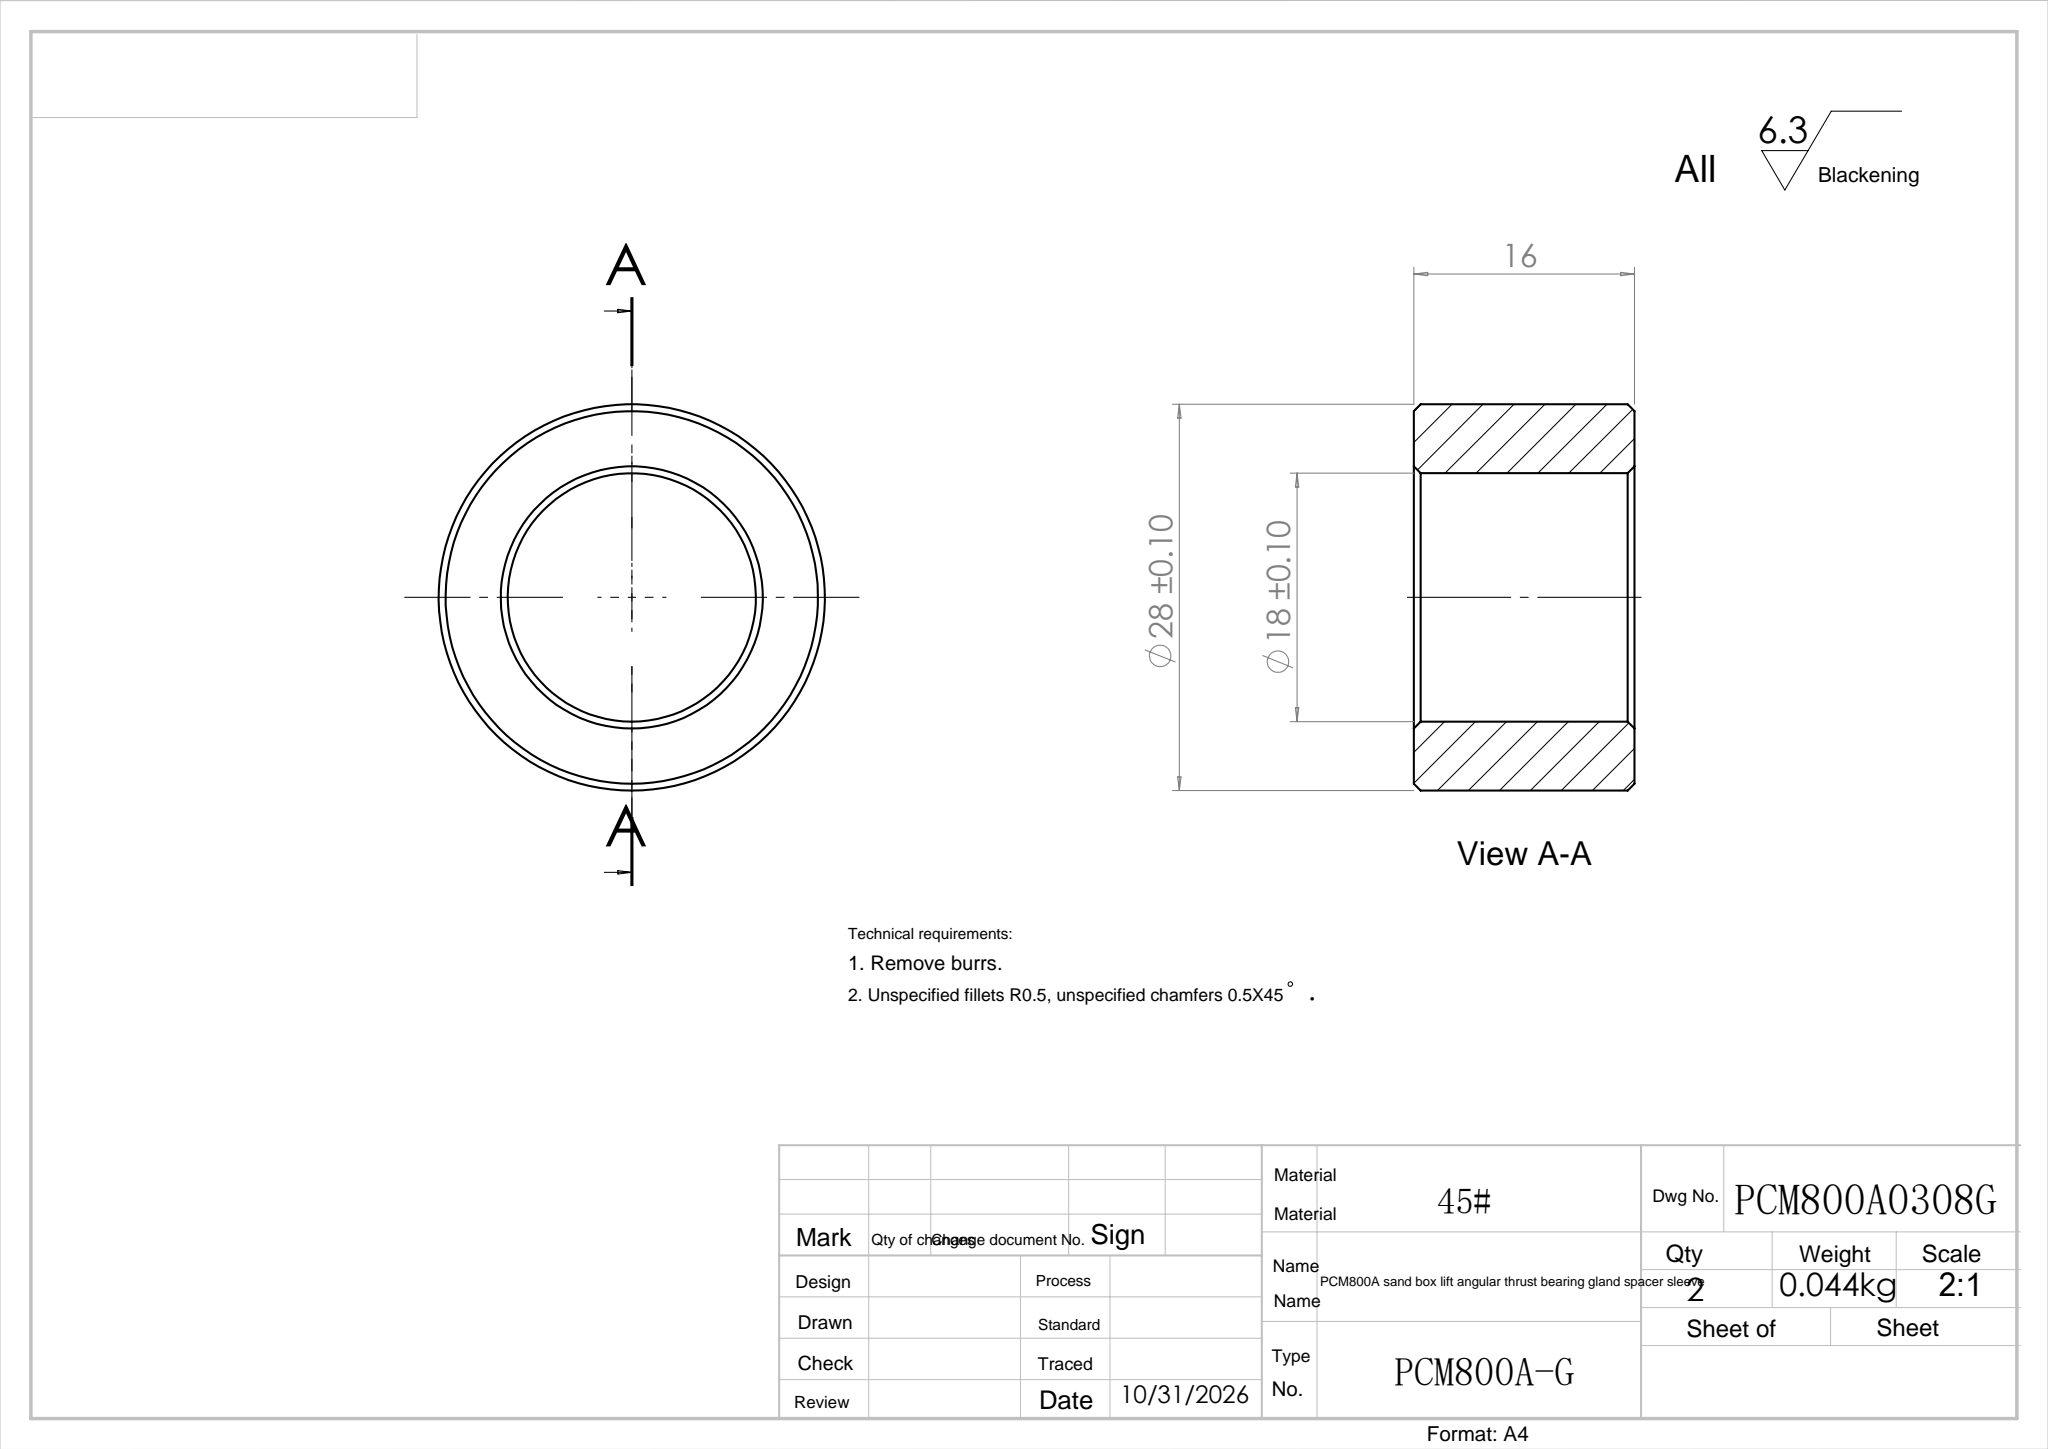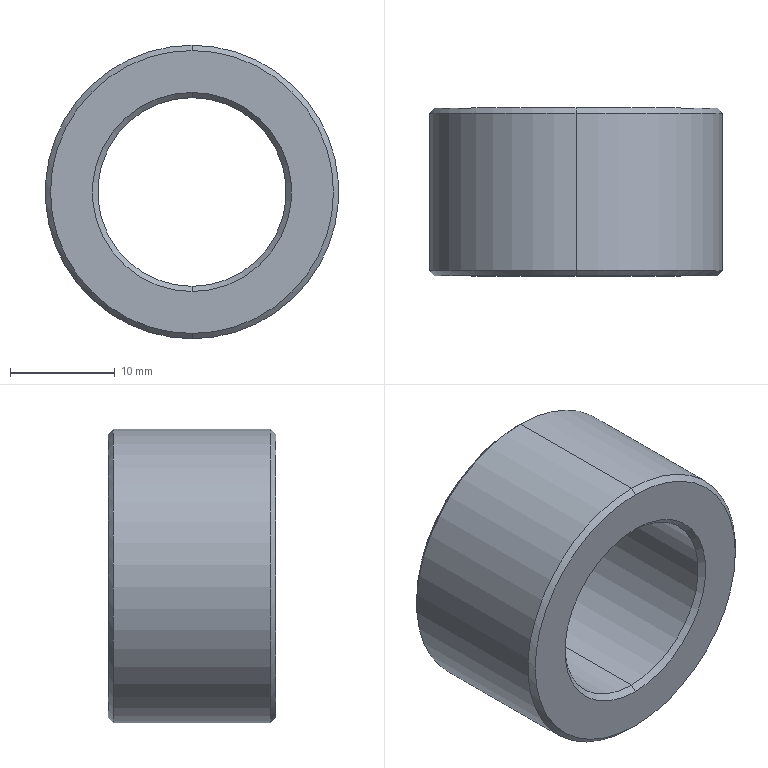Part | SolidWorks | features Chamfer 1, Extrusion 1 | 1 solid | 14 faces | box 28 x 16 x 28 mm | volume 5744 mm3 | cone 8 | cylinder 4 | plane 2 | commonest cylinder face diameters 18 x2 28 x2
STEP:
#1=CARTESIAN_POINT('',(0.,15.5,-9.));
#2=VERTEX_POINT('',#1);
#3=CARTESIAN_POINT('',(0.,15.5,9.));
#4=VERTEX_POINT('',#3);
#5=CARTESIAN_POINT('',(0.,15.5,0.));
#6=DIRECTION('',(0.,1.,0.));
#7=DIRECTION('',(0.,0.,1.));
#8=AXIS2_PLACEMENT_3D('',#5,#6,#7);
#9=CIRCLE('',#8,9.);
#10=EDGE_CURVE('',#2,#4,#9,.T.);
#11=ORIENTED_EDGE('',*,*,#10,.F.);
#12=CARTESIAN_POINT('',(0.,16.,-9.5));
#13=VERTEX_POINT('',#12);
#14=CARTESIAN_POINT('',(0.,15.5,-9.));
#15=DIRECTION('',(0.,0.7071,-0.7071));
#16=VECTOR('',#15,1000.);
#17=LINE('',#14,#16);
#18=EDGE_CURVE('',#2,#13,#17,.T.);
#19=ORIENTED_EDGE('',*,*,#18,.T.);
#20=CARTESIAN_POINT('',(0.,16.,9.5));
#21=VERTEX_POINT('',#20);
#22=CARTESIAN_POINT('',(0.,16.,0.));
#23=DIRECTION('',(0.,-1.,0.));
#24=DIRECTION('',(0.,0.,1.));
#25=AXIS2_PLACEMENT_3D('',#22,#23,#24);
#26=CIRCLE('',#25,9.5);
#27=EDGE_CURVE('',#21,#13,#26,.T.);
#28=ORIENTED_EDGE('',*,*,#27,.F.);
#29=CARTESIAN_POINT('',(0.,15.5,9.));
#30=DIRECTION('',(0.,0.7071,0.7071));
#31=VECTOR('',#30,1000.);
#32=LINE('',#29,#31);
#33=EDGE_CURVE('',#4,#21,#32,.T.);
#34=ORIENTED_EDGE('',*,*,#33,.F.);
#35=EDGE_LOOP('',(#11,#19,#28,#34));
#36=FACE_OUTER_BOUND('',#35,.T.);
#37=CARTESIAN_POINT('',(0.,15.5,0.));
#38=DIRECTION('',(0.,1.,0.));
#39=DIRECTION('',(0.,0.,1.));
#40=AXIS2_PLACEMENT_3D('',#37,#38,#39);
#41=CONICAL_SURFACE('',#40,9.,0.7854);
#42=ADVANCED_FACE('',(#36),#41,.F.);
#43=CARTESIAN_POINT('',(0.,16.,13.5));
#44=VERTEX_POINT('',#43);
#45=CARTESIAN_POINT('',(0.,16.,-13.5));
#46=VERTEX_POINT('',#45);
#47=CARTESIAN_POINT('',(0.,16.,0.));
#48=DIRECTION('',(0.,1.,0.));
#49=DIRECTION('',(0.,0.,1.));
#50=AXIS2_PLACEMENT_3D('',#47,#48,#49);
#51=CIRCLE('',#50,13.5);
#52=EDGE_CURVE('',#44,#46,#51,.T.);
#53=ORIENTED_EDGE('',*,*,#52,.F.);
#54=CARTESIAN_POINT('',(0.,15.5,14.));
#55=VERTEX_POINT('',#54);
#56=CARTESIAN_POINT('',(0.,16.,13.5));
#57=DIRECTION('',(0.,-0.7071,0.7071));
#58=VECTOR('',#57,1000.);
#59=LINE('',#56,#58);
#60=EDGE_CURVE('',#44,#55,#59,.T.);
#61=ORIENTED_EDGE('',*,*,#60,.T.);
#62=CARTESIAN_POINT('',(0.,15.5,-14.));
#63=VERTEX_POINT('',#62);
#64=CARTESIAN_POINT('',(0.,15.5,0.));
#65=DIRECTION('',(0.,-1.,0.));
#66=DIRECTION('',(0.,0.,1.));
#67=AXIS2_PLACEMENT_3D('',#64,#65,#66);
#68=CIRCLE('',#67,14.);
#69=EDGE_CURVE('',#63,#55,#68,.T.);
#70=ORIENTED_EDGE('',*,*,#69,.F.);
#71=CARTESIAN_POINT('',(0.,16.,-13.5));
#72=DIRECTION('',(0.,-0.7071,-0.7071));
#73=VECTOR('',#72,1000.);
#74=LINE('',#71,#73);
#75=EDGE_CURVE('',#46,#63,#74,.T.);
#76=ORIENTED_EDGE('',*,*,#75,.F.);
#77=EDGE_LOOP('',(#53,#61,#70,#76));
#78=FACE_OUTER_BOUND('',#77,.T.);
#79=CARTESIAN_POINT('',(0.,16.,0.));
#80=DIRECTION('',(0.,-1.,0.));
#81=DIRECTION('',(0.,0.,-1.));
#82=AXIS2_PLACEMENT_3D('',#79,#80,#81);
#83=CONICAL_SURFACE('',#82,13.5,0.7854);
#84=ADVANCED_FACE('',(#78),#83,.T.);
#85=CARTESIAN_POINT('',(0.,0.,-13.5));
#86=VERTEX_POINT('',#85);
#87=CARTESIAN_POINT('',(0.,0.,13.5));
#88=VERTEX_POINT('',#87);
#89=CARTESIAN_POINT('',(0.,0.,0.));
#90=DIRECTION('',(0.,-1.,0.));
#91=DIRECTION('',(0.,0.,1.));
#92=AXIS2_PLACEMENT_3D('',#89,#90,#91);
#93=CIRCLE('',#92,13.5);
#94=EDGE_CURVE('',#86,#88,#93,.T.);
#95=ORIENTED_EDGE('',*,*,#94,.F.);
#96=CARTESIAN_POINT('',(0.,0.5,-14.));
#97=VERTEX_POINT('',#96);
#98=CARTESIAN_POINT('',(0.,0.5,-14.));
#99=DIRECTION('',(0.,0.7071,-0.7071));
#100=VECTOR('',#99,1000.);
#101=LINE('',#98,#100);
#102=EDGE_CURVE('',#86,#97,#101,.T.);
#103=ORIENTED_EDGE('',*,*,#102,.T.);
#104=CARTESIAN_POINT('',(0.,0.5,14.));
#105=VERTEX_POINT('',#104);
#106=CARTESIAN_POINT('',(0.,0.5,0.));
#107=DIRECTION('',(0.,1.,0.));
#108=DIRECTION('',(0.,0.,1.));
#109=AXIS2_PLACEMENT_3D('',#106,#107,#108);
#110=CIRCLE('',#109,14.);
#111=EDGE_CURVE('',#105,#97,#110,.T.);
#112=ORIENTED_EDGE('',*,*,#111,.F.);
#113=CARTESIAN_POINT('',(0.,0.5,14.));
#114=DIRECTION('',(0.,0.7071,0.7071));
#115=VECTOR('',#114,1000.);
#116=LINE('',#113,#115);
#117=EDGE_CURVE('',#88,#105,#116,.T.);
#118=ORIENTED_EDGE('',*,*,#117,.F.);
#119=EDGE_LOOP('',(#95,#103,#112,#118));
#120=FACE_OUTER_BOUND('',#119,.T.);
#121=CARTESIAN_POINT('',(0.,0.5,0.));
#122=DIRECTION('',(0.,1.,0.));
#123=DIRECTION('',(0.,0.,1.));
#124=AXIS2_PLACEMENT_3D('',#121,#122,#123);
#125=CONICAL_SURFACE('',#124,14.,0.7854);
#126=ADVANCED_FACE('',(#120),#125,.T.);
#127=CARTESIAN_POINT('',(0.,0.5,9.));
#128=VERTEX_POINT('',#127);
#129=CARTESIAN_POINT('',(0.,0.5,-9.));
#130=VERTEX_POINT('',#129);
#131=CARTESIAN_POINT('',(0.,0.5,0.));
#132=DIRECTION('',(0.,-1.,0.));
#133=DIRECTION('',(0.,0.,1.));
#134=AXIS2_PLACEMENT_3D('',#131,#132,#133);
#135=CIRCLE('',#134,9.);
#136=EDGE_CURVE('',#128,#130,#135,.T.);
#137=ORIENTED_EDGE('',*,*,#136,.F.);
#138=CARTESIAN_POINT('',(0.,0.,9.5));
#139=VERTEX_POINT('',#138);
#140=CARTESIAN_POINT('',(0.,0.,9.5));
#141=DIRECTION('',(0.,-0.7071,0.7071));
#142=VECTOR('',#141,1000.);
#143=LINE('',#140,#142);
#144=EDGE_CURVE('',#128,#139,#143,.T.);
#145=ORIENTED_EDGE('',*,*,#144,.T.);
#146=CARTESIAN_POINT('',(0.,0.,-9.5));
#147=VERTEX_POINT('',#146);
#148=CARTESIAN_POINT('',(0.,0.,0.));
#149=DIRECTION('',(0.,1.,0.));
#150=DIRECTION('',(0.,0.,1.));
#151=AXIS2_PLACEMENT_3D('',#148,#149,#150);
#152=CIRCLE('',#151,9.5);
#153=EDGE_CURVE('',#147,#139,#152,.T.);
#154=ORIENTED_EDGE('',*,*,#153,.F.);
#155=CARTESIAN_POINT('',(0.,0.,-9.5));
#156=DIRECTION('',(0.,-0.7071,-0.7071));
#157=VECTOR('',#156,1000.);
#158=LINE('',#155,#157);
#159=EDGE_CURVE('',#130,#147,#158,.T.);
#160=ORIENTED_EDGE('',*,*,#159,.F.);
#161=EDGE_LOOP('',(#137,#145,#154,#160));
#162=FACE_OUTER_BOUND('',#161,.T.);
#163=CARTESIAN_POINT('',(0.,0.,0.));
#164=DIRECTION('',(0.,-1.,0.));
#165=DIRECTION('',(0.,0.,-1.));
#166=AXIS2_PLACEMENT_3D('',#163,#164,#165);
#167=CONICAL_SURFACE('',#166,9.5,0.7854);
#168=ADVANCED_FACE('',(#162),#167,.F.);
#169=ORIENTED_EDGE('',*,*,#10,.T.);
#170=CARTESIAN_POINT('',(0.,16.,9.));
#171=DIRECTION('',(0.,-1.,0.));
#172=VECTOR('',#171,1000.);
#173=LINE('',#170,#172);
#174=EDGE_CURVE('',#4,#128,#173,.T.);
#175=ORIENTED_EDGE('',*,*,#174,.T.);
#176=ORIENTED_EDGE('',*,*,#136,.T.);
#177=CARTESIAN_POINT('',(0.,16.,-9.));
#178=DIRECTION('',(0.,-1.,0.));
#179=VECTOR('',#178,1000.);
#180=LINE('',#177,#179);
#181=EDGE_CURVE('',#2,#130,#180,.T.);
#182=ORIENTED_EDGE('',*,*,#181,.F.);
#183=EDGE_LOOP('',(#169,#175,#176,#182));
#184=FACE_OUTER_BOUND('',#183,.T.);
#185=CARTESIAN_POINT('',(0.,16.,0.));
#186=DIRECTION('',(0.,-1.,0.));
#187=DIRECTION('',(0.,0.,-1.));
#188=AXIS2_PLACEMENT_3D('',#185,#186,#187);
#189=CYLINDRICAL_SURFACE('',#188,9.);
#190=ADVANCED_FACE('',(#184),#189,.F.);
#191=ORIENTED_EDGE('',*,*,#69,.T.);
#192=CARTESIAN_POINT('',(0.,16.,14.));
#193=DIRECTION('',(0.,-1.,0.));
#194=VECTOR('',#193,1000.);
#195=LINE('',#192,#194);
#196=EDGE_CURVE('',#55,#105,#195,.T.);
#197=ORIENTED_EDGE('',*,*,#196,.T.);
#198=ORIENTED_EDGE('',*,*,#111,.T.);
#199=CARTESIAN_POINT('',(0.,16.,-14.));
#200=DIRECTION('',(0.,-1.,0.));
#201=VECTOR('',#200,1000.);
#202=LINE('',#199,#201);
#203=EDGE_CURVE('',#63,#97,#202,.T.);
#204=ORIENTED_EDGE('',*,*,#203,.F.);
#205=EDGE_LOOP('',(#191,#197,#198,#204));
#206=FACE_OUTER_BOUND('',#205,.T.);
#207=CARTESIAN_POINT('',(0.,16.,0.));
#208=DIRECTION('',(0.,-1.,0.));
#209=DIRECTION('',(0.,0.,-1.));
#210=AXIS2_PLACEMENT_3D('',#207,#208,#209);
#211=CYLINDRICAL_SURFACE('',#210,14.);
#212=ADVANCED_FACE('',(#206),#211,.T.);
#213=CARTESIAN_POINT('',(0.,16.,0.));
#214=DIRECTION('',(0.,1.,0.));
#215=DIRECTION('',(0.,0.,1.));
#216=AXIS2_PLACEMENT_3D('',#213,#214,#215);
#217=CIRCLE('',#216,13.5);
#218=EDGE_CURVE('',#46,#44,#217,.T.);
#219=ORIENTED_EDGE('',*,*,#218,.T.);
#220=ORIENTED_EDGE('',*,*,#52,.T.);
#221=EDGE_LOOP('',(#219,#220));
#222=FACE_OUTER_BOUND('',#221,.T.);
#223=ORIENTED_EDGE('',*,*,#27,.T.);
#224=CARTESIAN_POINT('',(0.,16.,0.));
#225=DIRECTION('',(0.,-1.,0.));
#226=DIRECTION('',(0.,0.,1.));
#227=AXIS2_PLACEMENT_3D('',#224,#225,#226);
#228=CIRCLE('',#227,9.5);
#229=EDGE_CURVE('',#13,#21,#228,.T.);
#230=ORIENTED_EDGE('',*,*,#229,.T.);
#231=EDGE_LOOP('',(#223,#230));
#232=FACE_BOUND('',#231,.T.);
#233=CARTESIAN_POINT('',(0.,16.,0.));
#234=DIRECTION('',(0.,1.,0.));
#235=DIRECTION('',(0.,0.,1.));
#236=AXIS2_PLACEMENT_3D('',#233,#234,#235);
#237=PLANE('',#236);
#238=ADVANCED_FACE('',(#222,#232),#237,.T.);
#239=ORIENTED_EDGE('',*,*,#153,.T.);
#240=CARTESIAN_POINT('',(0.,0.,0.));
#241=DIRECTION('',(0.,1.,0.));
#242=DIRECTION('',(0.,0.,1.));
#243=AXIS2_PLACEMENT_3D('',#240,#241,#242);
#244=CIRCLE('',#243,9.5);
#245=EDGE_CURVE('',#139,#147,#244,.T.);
#246=ORIENTED_EDGE('',*,*,#245,.T.);
#247=EDGE_LOOP('',(#239,#246));
#248=FACE_BOUND('',#247,.T.);
#249=CARTESIAN_POINT('',(0.,0.,0.));
#250=DIRECTION('',(0.,-1.,0.));
#251=DIRECTION('',(0.,0.,1.));
#252=AXIS2_PLACEMENT_3D('',#249,#250,#251);
#253=CIRCLE('',#252,13.5);
#254=EDGE_CURVE('',#88,#86,#253,.T.);
#255=ORIENTED_EDGE('',*,*,#254,.T.);
#256=ORIENTED_EDGE('',*,*,#94,.T.);
#257=EDGE_LOOP('',(#255,#256));
#258=FACE_OUTER_BOUND('',#257,.T.);
#259=CARTESIAN_POINT('',(0.,0.,0.));
#260=DIRECTION('',(0.,1.,0.));
#261=DIRECTION('',(0.,0.,1.));
#262=AXIS2_PLACEMENT_3D('',#259,#260,#261);
#263=PLANE('',#262);
#264=ADVANCED_FACE('',(#248,#258),#263,.F.);
#265=ORIENTED_EDGE('',*,*,#196,.F.);
#266=CARTESIAN_POINT('',(0.,15.5,0.));
#267=DIRECTION('',(0.,-1.,0.));
#268=DIRECTION('',(0.,0.,1.));
#269=AXIS2_PLACEMENT_3D('',#266,#267,#268);
#270=CIRCLE('',#269,14.);
#271=EDGE_CURVE('',#55,#63,#270,.T.);
#272=ORIENTED_EDGE('',*,*,#271,.T.);
#273=ORIENTED_EDGE('',*,*,#203,.T.);
#274=CARTESIAN_POINT('',(0.,0.5,0.));
#275=DIRECTION('',(0.,1.,0.));
#276=DIRECTION('',(0.,0.,1.));
#277=AXIS2_PLACEMENT_3D('',#274,#275,#276);
#278=CIRCLE('',#277,14.);
#279=EDGE_CURVE('',#97,#105,#278,.T.);
#280=ORIENTED_EDGE('',*,*,#279,.T.);
#281=EDGE_LOOP('',(#265,#272,#273,#280));
#282=FACE_OUTER_BOUND('',#281,.T.);
#283=CARTESIAN_POINT('',(0.,16.,0.));
#284=DIRECTION('',(0.,-1.,0.));
#285=DIRECTION('',(0.,0.,-1.));
#286=AXIS2_PLACEMENT_3D('',#283,#284,#285);
#287=CYLINDRICAL_SURFACE('',#286,14.);
#288=ADVANCED_FACE('',(#282),#287,.T.);
#289=ORIENTED_EDGE('',*,*,#174,.F.);
#290=CARTESIAN_POINT('',(0.,15.5,0.));
#291=DIRECTION('',(0.,1.,0.));
#292=DIRECTION('',(0.,0.,1.));
#293=AXIS2_PLACEMENT_3D('',#290,#291,#292);
#294=CIRCLE('',#293,9.);
#295=EDGE_CURVE('',#4,#2,#294,.T.);
#296=ORIENTED_EDGE('',*,*,#295,.T.);
#297=ORIENTED_EDGE('',*,*,#181,.T.);
#298=CARTESIAN_POINT('',(0.,0.5,0.));
#299=DIRECTION('',(0.,-1.,0.));
#300=DIRECTION('',(0.,0.,1.));
#301=AXIS2_PLACEMENT_3D('',#298,#299,#300);
#302=CIRCLE('',#301,9.);
#303=EDGE_CURVE('',#130,#128,#302,.T.);
#304=ORIENTED_EDGE('',*,*,#303,.T.);
#305=EDGE_LOOP('',(#289,#296,#297,#304));
#306=FACE_OUTER_BOUND('',#305,.T.);
#307=CARTESIAN_POINT('',(0.,16.,0.));
#308=DIRECTION('',(0.,-1.,0.));
#309=DIRECTION('',(0.,0.,-1.));
#310=AXIS2_PLACEMENT_3D('',#307,#308,#309);
#311=CYLINDRICAL_SURFACE('',#310,9.);
#312=ADVANCED_FACE('',(#306),#311,.F.);
#313=ORIENTED_EDGE('',*,*,#144,.F.);
#314=ORIENTED_EDGE('',*,*,#303,.F.);
#315=ORIENTED_EDGE('',*,*,#159,.T.);
#316=ORIENTED_EDGE('',*,*,#245,.F.);
#317=EDGE_LOOP('',(#313,#314,#315,#316));
#318=FACE_OUTER_BOUND('',#317,.T.);
#319=CARTESIAN_POINT('',(0.,0.,0.));
#320=DIRECTION('',(0.,-1.,0.));
#321=DIRECTION('',(0.,0.,-1.));
#322=AXIS2_PLACEMENT_3D('',#319,#320,#321);
#323=CONICAL_SURFACE('',#322,9.5,0.7854);
#324=ADVANCED_FACE('',(#318),#323,.F.);
#325=ORIENTED_EDGE('',*,*,#102,.F.);
#326=ORIENTED_EDGE('',*,*,#254,.F.);
#327=ORIENTED_EDGE('',*,*,#117,.T.);
#328=ORIENTED_EDGE('',*,*,#279,.F.);
#329=EDGE_LOOP('',(#325,#326,#327,#328));
#330=FACE_OUTER_BOUND('',#329,.T.);
#331=CARTESIAN_POINT('',(0.,0.5,0.));
#332=DIRECTION('',(0.,1.,0.));
#333=DIRECTION('',(0.,0.,1.));
#334=AXIS2_PLACEMENT_3D('',#331,#332,#333);
#335=CONICAL_SURFACE('',#334,14.,0.7854);
#336=ADVANCED_FACE('',(#330),#335,.T.);
#337=ORIENTED_EDGE('',*,*,#60,.F.);
#338=ORIENTED_EDGE('',*,*,#218,.F.);
#339=ORIENTED_EDGE('',*,*,#75,.T.);
#340=ORIENTED_EDGE('',*,*,#271,.F.);
#341=EDGE_LOOP('',(#337,#338,#339,#340));
#342=FACE_OUTER_BOUND('',#341,.T.);
#343=CARTESIAN_POINT('',(0.,16.,0.));
#344=DIRECTION('',(0.,-1.,0.));
#345=DIRECTION('',(0.,0.,-1.));
#346=AXIS2_PLACEMENT_3D('',#343,#344,#345);
#347=CONICAL_SURFACE('',#346,13.5,0.7854);
#348=ADVANCED_FACE('',(#342),#347,.T.);
#349=ORIENTED_EDGE('',*,*,#18,.F.);
#350=ORIENTED_EDGE('',*,*,#295,.F.);
#351=ORIENTED_EDGE('',*,*,#33,.T.);
#352=ORIENTED_EDGE('',*,*,#229,.F.);
#353=EDGE_LOOP('',(#349,#350,#351,#352));
#354=FACE_OUTER_BOUND('',#353,.T.);
#355=CARTESIAN_POINT('',(0.,15.5,0.));
#356=DIRECTION('',(0.,1.,0.));
#357=DIRECTION('',(0.,0.,1.));
#358=AXIS2_PLACEMENT_3D('',#355,#356,#357);
#359=CONICAL_SURFACE('',#358,9.,0.7854);
#360=ADVANCED_FACE('',(#354),#359,.F.);
#361=CLOSED_SHELL('',(#42,#84,#126,#168,#190,#212,#238,#264,#288,#312,#324,#336,#348,#360));
#362=MANIFOLD_SOLID_BREP('',#361);
#363=CARTESIAN_POINT('',(0.,0.,0.));
#364=DIRECTION('',(0.,0.,1.));
#365=DIRECTION('',(1.,0.,0.));
#366=AXIS2_PLACEMENT_3D('',#363,#364,#365);
#367=(LENGTH_UNIT()NAMED_UNIT(*)SI_UNIT(.MILLI.,.METRE.));
#368=UNCERTAINTY_MEASURE_WITH_UNIT(LENGTH_MEASURE(0.00001),#367,'','');
#369=(NAMED_UNIT(*)PLANE_ANGLE_UNIT()SI_UNIT($,.RADIAN.));
#370=(NAMED_UNIT(*)SI_UNIT($,.STERADIAN.)SOLID_ANGLE_UNIT());
#371=(GEOMETRIC_REPRESENTATION_CONTEXT(3)GLOBAL_UNCERTAINTY_ASSIGNED_CONTEXT((#368))GLOBAL_UNIT_ASSIGNED_CONTEXT((#367,#369,#370))REPRESENTATION_CONTEXT('',''));
#372=ADVANCED_BREP_SHAPE_REPRESENTATION('',(#362,#366),#371);